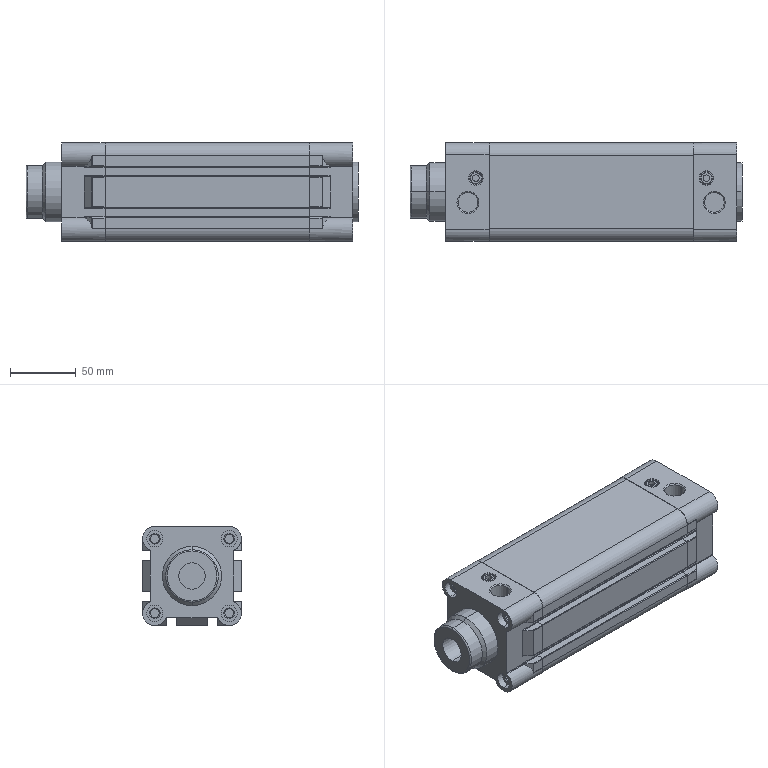Part | SolidWorks | features BaseBody 1 | 1 solid | 398 faces | box 252 x 75 x 75 mm | volume 699508 mm3 | cylinder 190 | plane 176 | cone 30 | torus 2 | commonest cylinder face diameters 1 x102 20 x18 6.647 x16 12.4 x16 18.5 x10 5 x4